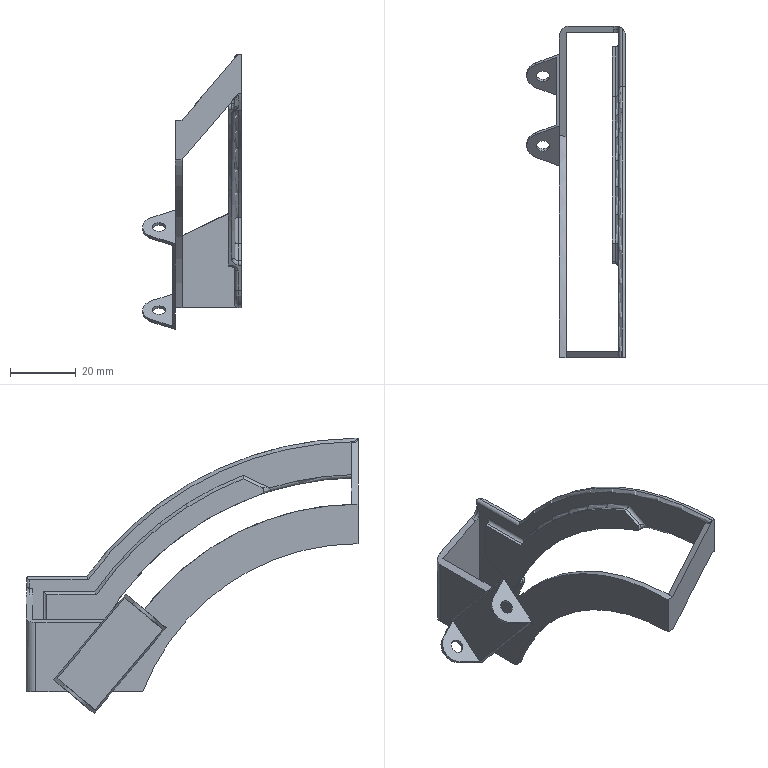Part | STEP file | Blade v2 | 1 solid | 83 faces | box 30 x 100.889 x 83.611 mm | volume 9239 mm3 | plane 37 | cylinder 34 | torus 7 | spline 5 | commonest cylinder face diameters 2 x18 4 x4 6 x3 10 x2 16 x1 140 x1